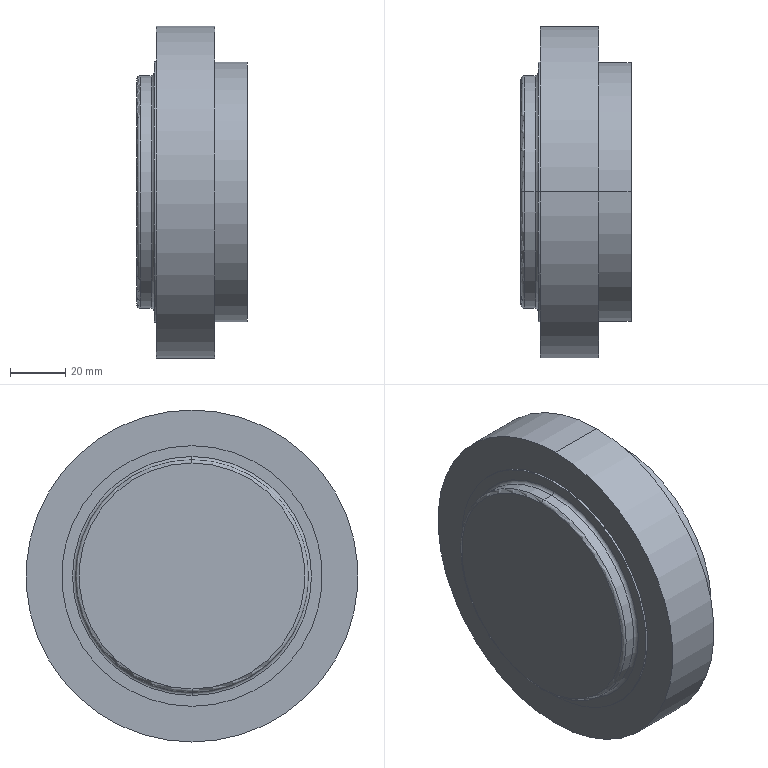Part | STEP file | Bearing end cap 1 | 1 solid | 26 faces | box 39.936 x 120.436 x 120.436 mm | volume 192561 mm3 | cylinder 10 | torus 6 | plane 6 | cone 4 | commonest cylinder face diameters 84.344 x2 87.483 x2 94.152 x2 94.544 x2 120.436 x2
STEP:
#1=CARTESIAN_POINT('',(-14.13,0.,40.292));
#2=VERTEX_POINT('',#1);
#3=CARTESIAN_POINT('',(-14.13,0.,-40.292));
#4=VERTEX_POINT('',#3);
#5=CARTESIAN_POINT('',(-14.13,0.,0.));
#6=DIRECTION('',(-1.,0.,0.));
#7=DIRECTION('',(0.,0.,1.));
#8=AXIS2_PLACEMENT_3D('',#5,#6,#7);
#9=CIRCLE('',#8,40.292);
#10=EDGE_CURVE('',#2,#4,#9,.T.);
#11=ORIENTED_EDGE('',*,*,#10,.F.);
#12=CARTESIAN_POINT('',(-15.049,0.,40.033));
#13=VERTEX_POINT('',#12);
#14=CARTESIAN_POINT('',(-15.644,0.,43.911));
#15=DIRECTION('',(0.,1.,0.));
#16=DIRECTION('',(0.,0.,1.));
#17=AXIS2_PLACEMENT_3D('',#14,#15,#16);
#18=CIRCLE('',#17,3.923);
#19=EDGE_CURVE('',#2,#13,#18,.T.);
#20=ORIENTED_EDGE('',*,*,#19,.T.);
#21=CARTESIAN_POINT('',(-15.049,0.,-40.033));
#22=VERTEX_POINT('',#21);
#23=CARTESIAN_POINT('',(-15.049,0.,0.));
#24=DIRECTION('',(1.,0.,0.));
#25=DIRECTION('',(0.,0.,1.));
#26=AXIS2_PLACEMENT_3D('',#23,#24,#25);
#27=CIRCLE('',#26,40.033);
#28=EDGE_CURVE('',#22,#13,#27,.T.);
#29=ORIENTED_EDGE('',*,*,#28,.F.);
#30=CARTESIAN_POINT('',(-15.644,0.,-43.911));
#31=DIRECTION('',(0.,-1.,0.));
#32=DIRECTION('',(0.,0.,-1.));
#33=AXIS2_PLACEMENT_3D('',#30,#31,#32);
#34=CIRCLE('',#33,3.923);
#35=EDGE_CURVE('',#4,#22,#34,.T.);
#36=ORIENTED_EDGE('',*,*,#35,.F.);
#37=EDGE_LOOP('',(#11,#20,#29,#36));
#38=FACE_OUTER_BOUND('',#37,.T.);
#39=CARTESIAN_POINT('',(-15.644,0.,0.));
#40=DIRECTION('',(1.,0.,0.));
#41=DIRECTION('',(0.,0.,-1.));
#42=AXIS2_PLACEMENT_3D('',#39,#40,#41);
#43=TOROIDAL_SURFACE('',#42,43.911,3.923);
#44=ADVANCED_FACE('',(#38),#43,.T.);
#45=CARTESIAN_POINT('',(-39.936,0.,40.995));
#46=VERTEX_POINT('',#45);
#47=CARTESIAN_POINT('',(-39.936,0.,-40.995));
#48=VERTEX_POINT('',#47);
#49=CARTESIAN_POINT('',(-39.936,0.,0.));
#50=DIRECTION('',(-1.,0.,0.));
#51=DIRECTION('',(0.,0.,-1.));
#52=AXIS2_PLACEMENT_3D('',#49,#50,#51);
#53=CIRCLE('',#52,40.995);
#54=EDGE_CURVE('',#46,#48,#53,.T.);
#55=ORIENTED_EDGE('',*,*,#54,.F.);
#56=CARTESIAN_POINT('',(-38.759,0.,42.172));
#57=VERTEX_POINT('',#56);
#58=CARTESIAN_POINT('',(-38.759,0.,40.995));
#59=DIRECTION('',(0.,1.,0.));
#60=DIRECTION('',(0.,0.,1.));
#61=AXIS2_PLACEMENT_3D('',#58,#59,#60);
#62=CIRCLE('',#61,1.177);
#63=EDGE_CURVE('',#46,#57,#62,.T.);
#64=ORIENTED_EDGE('',*,*,#63,.T.);
#65=CARTESIAN_POINT('',(-38.759,0.,-42.172));
#66=VERTEX_POINT('',#65);
#67=CARTESIAN_POINT('',(-38.759,0.,0.));
#68=DIRECTION('',(1.,0.,0.));
#69=DIRECTION('',(0.,0.,-1.));
#70=AXIS2_PLACEMENT_3D('',#67,#68,#69);
#71=CIRCLE('',#70,42.172);
#72=EDGE_CURVE('',#66,#57,#71,.T.);
#73=ORIENTED_EDGE('',*,*,#72,.F.);
#74=CARTESIAN_POINT('',(-38.759,0.,-40.995));
#75=DIRECTION('',(0.,-1.,0.));
#76=DIRECTION('',(0.,0.,-1.));
#77=AXIS2_PLACEMENT_3D('',#74,#75,#76);
#78=CIRCLE('',#77,1.177);
#79=EDGE_CURVE('',#48,#66,#78,.T.);
#80=ORIENTED_EDGE('',*,*,#79,.F.);
#81=EDGE_LOOP('',(#55,#64,#73,#80));
#82=FACE_OUTER_BOUND('',#81,.T.);
#83=CARTESIAN_POINT('',(-38.759,0.,0.));
#84=DIRECTION('',(1.,0.,0.));
#85=DIRECTION('',(0.,0.,-1.));
#86=AXIS2_PLACEMENT_3D('',#83,#84,#85);
#87=TOROIDAL_SURFACE('',#86,40.995,1.177);
#88=ADVANCED_FACE('',(#82),#87,.T.);
#89=CARTESIAN_POINT('',(-33.659,0.,43.349));
#90=VERTEX_POINT('',#89);
#91=CARTESIAN_POINT('',(-33.659,0.,-43.349));
#92=VERTEX_POINT('',#91);
#93=CARTESIAN_POINT('',(-33.659,0.,0.));
#94=DIRECTION('',(1.,0.,0.));
#95=DIRECTION('',(0.,0.,-1.));
#96=AXIS2_PLACEMENT_3D('',#93,#94,#95);
#97=CIRCLE('',#96,43.349);
#98=EDGE_CURVE('',#90,#92,#97,.T.);
#99=ORIENTED_EDGE('',*,*,#98,.F.);
#100=CARTESIAN_POINT('',(-34.836,0.,42.172));
#101=VERTEX_POINT('',#100);
#102=CARTESIAN_POINT('',(-34.836,0.,43.349));
#103=DIRECTION('',(0.,1.,0.));
#104=DIRECTION('',(0.,0.,1.));
#105=AXIS2_PLACEMENT_3D('',#102,#103,#104);
#106=CIRCLE('',#105,1.177);
#107=EDGE_CURVE('',#90,#101,#106,.T.);
#108=ORIENTED_EDGE('',*,*,#107,.T.);
#109=CARTESIAN_POINT('',(-34.836,0.,-42.172));
#110=VERTEX_POINT('',#109);
#111=CARTESIAN_POINT('',(-34.836,0.,0.));
#112=DIRECTION('',(-1.,0.,0.));
#113=DIRECTION('',(0.,0.,-1.));
#114=AXIS2_PLACEMENT_3D('',#111,#112,#113);
#115=CIRCLE('',#114,42.172);
#116=EDGE_CURVE('',#110,#101,#115,.T.);
#117=ORIENTED_EDGE('',*,*,#116,.F.);
#118=CARTESIAN_POINT('',(-34.836,0.,-43.349));
#119=DIRECTION('',(0.,-1.,0.));
#120=DIRECTION('',(0.,0.,-1.));
#121=AXIS2_PLACEMENT_3D('',#118,#119,#120);
#122=CIRCLE('',#121,1.177);
#123=EDGE_CURVE('',#92,#110,#122,.T.);
#124=ORIENTED_EDGE('',*,*,#123,.F.);
#125=EDGE_LOOP('',(#99,#108,#117,#124));
#126=FACE_OUTER_BOUND('',#125,.T.);
#127=CARTESIAN_POINT('',(-34.836,0.,0.));
#128=DIRECTION('',(1.,0.,0.));
#129=DIRECTION('',(0.,0.,-1.));
#130=AXIS2_PLACEMENT_3D('',#127,#128,#129);
#131=TOROIDAL_SURFACE('',#130,43.349,1.177);
#132=ADVANCED_FACE('',(#126),#131,.F.);
#133=CARTESIAN_POINT('',(-11.769,0.,60.218));
#134=VERTEX_POINT('',#133);
#135=CARTESIAN_POINT('',(-11.769,0.,-60.218));
#136=VERTEX_POINT('',#135);
#137=CARTESIAN_POINT('',(-11.769,0.,0.));
#138=DIRECTION('',(-1.,0.,0.));
#139=DIRECTION('',(0.,0.,1.));
#140=AXIS2_PLACEMENT_3D('',#137,#138,#139);
#141=CIRCLE('',#140,60.218);
#142=EDGE_CURVE('',#134,#136,#141,.T.);
#143=ORIENTED_EDGE('',*,*,#142,.T.);
#144=CARTESIAN_POINT('',(-32.875,0.,-60.218));
#145=VERTEX_POINT('',#144);
#146=CARTESIAN_POINT('',(0.,0.,-60.218));
#147=DIRECTION('',(-1.,0.,0.));
#148=VECTOR('',#147,1000.);
#149=LINE('',#146,#148);
#150=EDGE_CURVE('',#136,#145,#149,.T.);
#151=ORIENTED_EDGE('',*,*,#150,.T.);
#152=CARTESIAN_POINT('',(-32.875,0.,60.218));
#153=VERTEX_POINT('',#152);
#154=CARTESIAN_POINT('',(-32.875,0.,0.));
#155=DIRECTION('',(-1.,0.,0.));
#156=DIRECTION('',(0.,0.,1.));
#157=AXIS2_PLACEMENT_3D('',#154,#155,#156);
#158=CIRCLE('',#157,60.218);
#159=EDGE_CURVE('',#153,#145,#158,.T.);
#160=ORIENTED_EDGE('',*,*,#159,.F.);
#161=CARTESIAN_POINT('',(0.,0.,60.218));
#162=DIRECTION('',(-1.,0.,0.));
#163=VECTOR('',#162,1000.);
#164=LINE('',#161,#163);
#165=EDGE_CURVE('',#134,#153,#164,.T.);
#166=ORIENTED_EDGE('',*,*,#165,.F.);
#167=EDGE_LOOP('',(#143,#151,#160,#166));
#168=FACE_OUTER_BOUND('',#167,.T.);
#169=CARTESIAN_POINT('',(0.,0.,0.));
#170=DIRECTION('',(-1.,0.,0.));
#171=DIRECTION('',(0.,0.,1.));
#172=AXIS2_PLACEMENT_3D('',#169,#170,#171);
#173=CYLINDRICAL_SURFACE('',#172,60.218);
#174=ADVANCED_FACE('',(#168),#173,.T.);
#175=CARTESIAN_POINT('',(-32.875,0.,47.272));
#176=VERTEX_POINT('',#175);
#177=CARTESIAN_POINT('',(-32.875,0.,-47.272));
#178=VERTEX_POINT('',#177);
#179=CARTESIAN_POINT('',(-32.875,0.,0.));
#180=DIRECTION('',(-1.,0.,0.));
#181=DIRECTION('',(0.,0.,1.));
#182=AXIS2_PLACEMENT_3D('',#179,#180,#181);
#183=CIRCLE('',#182,47.272);
#184=EDGE_CURVE('',#176,#178,#183,.T.);
#185=ORIENTED_EDGE('',*,*,#184,.T.);
#186=CARTESIAN_POINT('',(-33.659,0.,-47.272));
#187=VERTEX_POINT('',#186);
#188=CARTESIAN_POINT('',(0.,0.,-47.272));
#189=DIRECTION('',(-1.,0.,0.));
#190=VECTOR('',#189,1000.);
#191=LINE('',#188,#190);
#192=EDGE_CURVE('',#178,#187,#191,.T.);
#193=ORIENTED_EDGE('',*,*,#192,.T.);
#194=CARTESIAN_POINT('',(-33.659,0.,47.272));
#195=VERTEX_POINT('',#194);
#196=CARTESIAN_POINT('',(-33.659,0.,0.));
#197=DIRECTION('',(-1.,0.,0.));
#198=DIRECTION('',(0.,0.,1.));
#199=AXIS2_PLACEMENT_3D('',#196,#197,#198);
#200=CIRCLE('',#199,47.272);
#201=EDGE_CURVE('',#195,#187,#200,.T.);
#202=ORIENTED_EDGE('',*,*,#201,.F.);
#203=CARTESIAN_POINT('',(0.,0.,47.272));
#204=DIRECTION('',(-1.,0.,0.));
#205=VECTOR('',#204,1000.);
#206=LINE('',#203,#205);
#207=EDGE_CURVE('',#176,#195,#206,.T.);
#208=ORIENTED_EDGE('',*,*,#207,.F.);
#209=EDGE_LOOP('',(#185,#193,#202,#208));
#210=FACE_OUTER_BOUND('',#209,.T.);
#211=CARTESIAN_POINT('',(0.,0.,0.));
#212=DIRECTION('',(-1.,0.,0.));
#213=DIRECTION('',(0.,0.,1.));
#214=AXIS2_PLACEMENT_3D('',#211,#212,#213);
#215=CYLINDRICAL_SURFACE('',#214,47.272);
#216=ADVANCED_FACE('',(#210),#215,.T.);
#217=CARTESIAN_POINT('',(-34.836,0.,0.));
#218=DIRECTION('',(-1.,0.,0.));
#219=DIRECTION('',(0.,0.,-1.));
#220=AXIS2_PLACEMENT_3D('',#217,#218,#219);
#221=CIRCLE('',#220,42.172);
#222=EDGE_CURVE('',#101,#110,#221,.T.);
#223=ORIENTED_EDGE('',*,*,#222,.T.);
#224=CARTESIAN_POINT('',(0.,0.,-42.172));
#225=DIRECTION('',(-1.,0.,0.));
#226=VECTOR('',#225,1000.);
#227=LINE('',#224,#226);
#228=EDGE_CURVE('',#110,#66,#227,.T.);
#229=ORIENTED_EDGE('',*,*,#228,.T.);
#230=ORIENTED_EDGE('',*,*,#72,.T.);
#231=CARTESIAN_POINT('',(0.,0.,42.172));
#232=DIRECTION('',(-1.,0.,0.));
#233=VECTOR('',#232,1000.);
#234=LINE('',#231,#233);
#235=EDGE_CURVE('',#101,#57,#234,.T.);
#236=ORIENTED_EDGE('',*,*,#235,.F.);
#237=EDGE_LOOP('',(#223,#229,#230,#236));
#238=FACE_OUTER_BOUND('',#237,.T.);
#239=CARTESIAN_POINT('',(0.,0.,0.));
#240=DIRECTION('',(-1.,0.,0.));
#241=DIRECTION('',(0.,0.,1.));
#242=AXIS2_PLACEMENT_3D('',#239,#240,#241);
#243=CYLINDRICAL_SURFACE('',#242,42.172);
#244=ADVANCED_FACE('',(#238),#243,.T.);
#245=CARTESIAN_POINT('',(-33.071,0.,-37.268));
#246=VERTEX_POINT('',#245);
#247=CARTESIAN_POINT('',(-33.071,0.,37.268));
#248=VERTEX_POINT('',#247);
#249=CARTESIAN_POINT('',(-33.071,0.,0.));
#250=DIRECTION('',(-1.,0.,0.));
#251=DIRECTION('',(0.,0.,1.));
#252=AXIS2_PLACEMENT_3D('',#249,#250,#251);
#253=CIRCLE('',#252,37.268);
#254=EDGE_CURVE('',#246,#248,#253,.T.);
#255=ORIENTED_EDGE('',*,*,#254,.T.);
#256=CARTESIAN_POINT('',(-33.071,0.,37.268));
#257=DIRECTION('',(0.9884,0.,0.1516));
#258=VECTOR('',#257,1000.);
#259=LINE('',#256,#258);
#260=EDGE_CURVE('',#248,#13,#259,.T.);
#261=ORIENTED_EDGE('',*,*,#260,.T.);
#262=CARTESIAN_POINT('',(-15.049,0.,0.));
#263=DIRECTION('',(1.,0.,0.));
#264=DIRECTION('',(0.,0.,1.));
#265=AXIS2_PLACEMENT_3D('',#262,#263,#264);
#266=CIRCLE('',#265,40.033);
#267=EDGE_CURVE('',#13,#22,#266,.T.);
#268=ORIENTED_EDGE('',*,*,#267,.T.);
#269=CARTESIAN_POINT('',(-33.071,0.,-37.268));
#270=DIRECTION('',(0.9884,0.,-0.1516));
#271=VECTOR('',#270,1000.);
#272=LINE('',#269,#271);
#273=EDGE_CURVE('',#246,#22,#272,.T.);
#274=ORIENTED_EDGE('',*,*,#273,.F.);
#275=EDGE_LOOP('',(#255,#261,#268,#274));
#276=FACE_OUTER_BOUND('',#275,.T.);
#277=CARTESIAN_POINT('',(-33.071,0.,0.));
#278=DIRECTION('',(1.,0.,0.));
#279=DIRECTION('',(0.,0.,-1.));
#280=AXIS2_PLACEMENT_3D('',#277,#278,#279);
#281=CONICAL_SURFACE('',#280,37.268,0.1522);
#282=ADVANCED_FACE('',(#276),#281,.F.);
#283=CARTESIAN_POINT('',(-14.13,0.,0.));
#284=DIRECTION('',(-1.,0.,0.));
#285=DIRECTION('',(0.,0.,1.));
#286=AXIS2_PLACEMENT_3D('',#283,#284,#285);
#287=CIRCLE('',#286,40.292);
#288=EDGE_CURVE('',#4,#2,#287,.T.);
#289=ORIENTED_EDGE('',*,*,#288,.T.);
#290=CARTESIAN_POINT('',(-5.884,0.,43.741));
#291=VERTEX_POINT('',#290);
#292=CARTESIAN_POINT('',(-14.574,0.,40.106));
#293=DIRECTION('',(0.9225,0.,0.386));
#294=VECTOR('',#293,1000.);
#295=LINE('',#292,#294);
#296=EDGE_CURVE('',#2,#291,#295,.T.);
#297=ORIENTED_EDGE('',*,*,#296,.T.);
#298=CARTESIAN_POINT('',(-5.884,0.,-43.741));
#299=VERTEX_POINT('',#298);
#300=CARTESIAN_POINT('',(-5.884,0.,0.));
#301=DIRECTION('',(-1.,0.,0.));
#302=DIRECTION('',(0.,0.,1.));
#303=AXIS2_PLACEMENT_3D('',#300,#301,#302);
#304=CIRCLE('',#303,43.741);
#305=EDGE_CURVE('',#299,#291,#304,.T.);
#306=ORIENTED_EDGE('',*,*,#305,.F.);
#307=CARTESIAN_POINT('',(-14.574,0.,-40.106));
#308=DIRECTION('',(0.9225,0.,-0.386));
#309=VECTOR('',#308,1000.);
#310=LINE('',#307,#309);
#311=EDGE_CURVE('',#4,#299,#310,.T.);
#312=ORIENTED_EDGE('',*,*,#311,.F.);
#313=EDGE_LOOP('',(#289,#297,#306,#312));
#314=FACE_OUTER_BOUND('',#313,.T.);
#315=CARTESIAN_POINT('',(-14.574,0.,0.));
#316=DIRECTION('',(1.,0.,0.));
#317=DIRECTION('',(0.,0.,-1.));
#318=AXIS2_PLACEMENT_3D('',#315,#316,#317);
#319=CONICAL_SURFACE('',#318,40.106,0.3962);
#320=ADVANCED_FACE('',(#314),#319,.F.);
#321=CARTESIAN_POINT('',(0.,0.,-43.741));
#322=VERTEX_POINT('',#321);
#323=CARTESIAN_POINT('',(0.,0.,43.741));
#324=VERTEX_POINT('',#323);
#325=CARTESIAN_POINT('',(0.,0.,0.));
#326=DIRECTION('',(-1.,0.,0.));
#327=DIRECTION('',(0.,0.,1.));
#328=AXIS2_PLACEMENT_3D('',#325,#326,#327);
#329=CIRCLE('',#328,43.741);
#330=EDGE_CURVE('',#322,#324,#329,.T.);
#331=ORIENTED_EDGE('',*,*,#330,.F.);
#332=CARTESIAN_POINT('',(0.,0.,-43.741));
#333=DIRECTION('',(-1.,0.,0.));
#334=VECTOR('',#333,1000.);
#335=LINE('',#332,#334);
#336=EDGE_CURVE('',#322,#299,#335,.T.);
#337=ORIENTED_EDGE('',*,*,#336,.T.);
#338=ORIENTED_EDGE('',*,*,#305,.T.);
#339=CARTESIAN_POINT('',(0.,0.,43.741));
#340=DIRECTION('',(-1.,0.,0.));
#341=VECTOR('',#340,1000.);
#342=LINE('',#339,#341);
#343=EDGE_CURVE('',#324,#291,#342,.T.);
#344=ORIENTED_EDGE('',*,*,#343,.F.);
#345=EDGE_LOOP('',(#331,#337,#338,#344));
#346=FACE_OUTER_BOUND('',#345,.T.);
#347=CARTESIAN_POINT('',(0.,0.,0.));
#348=DIRECTION('',(-1.,0.,0.));
#349=DIRECTION('',(0.,0.,1.));
#350=AXIS2_PLACEMENT_3D('',#347,#348,#349);
#351=CYLINDRICAL_SURFACE('',#350,43.741);
#352=ADVANCED_FACE('',(#346),#351,.F.);
#353=CARTESIAN_POINT('',(0.,0.,47.076));
#354=VERTEX_POINT('',#353);
#355=CARTESIAN_POINT('',(0.,0.,-47.076));
#356=VERTEX_POINT('',#355);
#357=CARTESIAN_POINT('',(0.,0.,0.));
#358=DIRECTION('',(-1.,0.,0.));
#359=DIRECTION('',(0.,0.,1.));
#360=AXIS2_PLACEMENT_3D('',#357,#358,#359);
#361=CIRCLE('',#360,47.076);
#362=EDGE_CURVE('',#354,#356,#361,.T.);
#363=ORIENTED_EDGE('',*,*,#362,.T.);
#364=CARTESIAN_POINT('',(-11.769,0.,-47.076));
#365=VERTEX_POINT('',#364);
#366=CARTESIAN_POINT('',(0.,0.,-47.076));
#367=DIRECTION('',(-1.,0.,0.));
#368=VECTOR('',#367,1000.);
#369=LINE('',#366,#368);
#370=EDGE_CURVE('',#356,#365,#369,.T.);
#371=ORIENTED_EDGE('',*,*,#370,.T.);
#372=CARTESIAN_POINT('',(-11.769,0.,47.076));
#373=VERTEX_POINT('',#372);
#374=CARTESIAN_POINT('',(-11.769,0.,0.));
#375=DIRECTION('',(-1.,0.,0.));
#376=DIRECTION('',(0.,0.,1.));
#377=AXIS2_PLACEMENT_3D('',#374,#375,#376);
#378=CIRCLE('',#377,47.076);
#379=EDGE_CURVE('',#373,#365,#378,.T.);
#380=ORIENTED_EDGE('',*,*,#379,.F.);
#381=CARTESIAN_POINT('',(0.,0.,47.076));
#382=DIRECTION('',(-1.,0.,0.));
#383=VECTOR('',#382,1000.);
#384=LINE('',#381,#383);
#385=EDGE_CURVE('',#354,#373,#384,.T.);
#386=ORIENTED_EDGE('',*,*,#385,.F.);
#387=EDGE_LOOP('',(#363,#371,#380,#386));
#388=FACE_OUTER_BOUND('',#387,.T.);
#389=CARTESIAN_POINT('',(0.,0.,0.));
#390=DIRECTION('',(-1.,0.,0.));
#391=DIRECTION('',(0.,0.,1.));
#392=AXIS2_PLACEMENT_3D('',#389,#390,#391);
#393=CYLINDRICAL_SURFACE('',#392,47.076);
#394=ADVANCED_FACE('',(#388),#393,.T.);
#395=ORIENTED_EDGE('',*,*,#370,.F.);
#396=CARTESIAN_POINT('',(0.,0.,0.));
#397=DIRECTION('',(-1.,0.,0.));
#398=DIRECTION('',(0.,0.,1.));
#399=AXIS2_PLACEMENT_3D('',#396,#397,#398);
#400=CIRCLE('',#399,47.076);
#401=EDGE_CURVE('',#356,#354,#400,.T.);
#402=ORIENTED_EDGE('',*,*,#401,.T.);
#403=ORIENTED_EDGE('',*,*,#385,.T.);
#404=CARTESIAN_POINT('',(-11.769,0.,0.));
#405=DIRECTION('',(-1.,0.,0.));
#406=DIRECTION('',(0.,0.,1.));
#407=AXIS2_PLACEMENT_3D('',#404,#405,#406);
#408=CIRCLE('',#407,47.076);
#409=EDGE_CURVE('',#365,#373,#408,.T.);
#410=ORIENTED_EDGE('',*,*,#409,.F.);
#411=EDGE_LOOP('',(#395,#402,#403,#410));
#412=FACE_OUTER_BOUND('',#411,.T.);
#413=CARTESIAN_POINT('',(0.,0.,0.));
#414=DIRECTION('',(-1.,0.,0.));
#415=DIRECTION('',(0.,0.,1.));
#416=AXIS2_PLACEMENT_3D('',#413,#414,#415);
#417=CYLINDRICAL_SURFACE('',#416,47.076);
#418=ADVANCED_FACE('',(#412),#417,.T.);
#419=ORIENTED_EDGE('',*,*,#362,.F.);
#420=ORIENTED_EDGE('',*,*,#401,.F.);
#421=EDGE_LOOP('',(#419,#420));
#422=FACE_OUTER_BOUND('',#421,.T.);
#423=CARTESIAN_POINT('',(0.,0.,0.));
#424=DIRECTION('',(-1.,0.,0.));
#425=DIRECTION('',(0.,0.,1.));
#426=AXIS2_PLACEMENT_3D('',#423,#424,#425);
#427=CIRCLE('',#426,43.741);
#428=EDGE_CURVE('',#324,#322,#427,.T.);
#429=ORIENTED_EDGE('',*,*,#428,.T.);
#430=ORIENTED_EDGE('',*,*,#330,.T.);
#431=EDGE_LOOP('',(#429,#430));
#432=FACE_BOUND('',#431,.T.);
#433=CARTESIAN_POINT('',(0.,47.076,0.));
#434=DIRECTION('',(-1.,0.,0.));
#435=DIRECTION('',(0.,0.,1.));
#436=AXIS2_PLACEMENT_3D('',#433,#434,#435);
#437=PLANE('',#436);
#438=ADVANCED_FACE('',(#422,#432),#437,.F.);
#439=ORIENTED_EDGE('',*,*,#336,.F.);
#440=ORIENTED_EDGE('',*,*,#428,.F.);
#441=ORIENTED_EDGE('',*,*,#343,.T.);
#442=CARTESIAN_POINT('',(-5.884,0.,0.));
#443=DIRECTION('',(-1.,0.,0.));
#444=DIRECTION('',(0.,0.,1.));
#445=AXIS2_PLACEMENT_3D('',#442,#443,#444);
#446=CIRCLE('',#445,43.741);
#447=EDGE_CURVE('',#291,#299,#446,.T.);
#448=ORIENTED_EDGE('',*,*,#447,.T.);
#449=EDGE_LOOP('',(#439,#440,#441,#448));
#450=FACE_OUTER_BOUND('',#449,.T.);
#451=CARTESIAN_POINT('',(0.,0.,0.));
#452=DIRECTION('',(-1.,0.,0.));
#453=DIRECTION('',(0.,0.,1.));
#454=AXIS2_PLACEMENT_3D('',#451,#452,#453);
#455=CYLINDRICAL_SURFACE('',#454,43.741);
#456=ADVANCED_FACE('',(#450),#455,.F.);
#457=ORIENTED_EDGE('',*,*,#296,.F.);
#458=ORIENTED_EDGE('',*,*,#10,.T.);
#459=ORIENTED_EDGE('',*,*,#311,.T.);
#460=ORIENTED_EDGE('',*,*,#447,.F.);
#461=EDGE_LOOP('',(#457,#458,#459,#460));
#462=FACE_OUTER_BOUND('',#461,.T.);
#463=CARTESIAN_POINT('',(-14.574,0.,0.));
#464=DIRECTION('',(1.,0.,0.));
#465=DIRECTION('',(0.,0.,-1.));
#466=AXIS2_PLACEMENT_3D('',#463,#464,#465);
#467=CONICAL_SURFACE('',#466,40.106,0.3962);
#468=ADVANCED_FACE('',(#462),#467,.F.);
#469=ORIENTED_EDGE('',*,*,#260,.F.);
#470=CARTESIAN_POINT('',(-33.071,0.,0.));
#471=DIRECTION('',(-1.,0.,0.));
#472=DIRECTION('',(0.,0.,1.));
#473=AXIS2_PLACEMENT_3D('',#470,#471,#472);
#474=CIRCLE('',#473,37.268);
#475=EDGE_CURVE('',#248,#246,#474,.T.);
#476=ORIENTED_EDGE('',*,*,#475,.T.);
#477=ORIENTED_EDGE('',*,*,#273,.T.);
#478=ORIENTED_EDGE('',*,*,#28,.T.);
#479=EDGE_LOOP('',(#469,#476,#477,#478));
#480=FACE_OUTER_BOUND('',#479,.T.);
#481=CARTESIAN_POINT('',(-33.071,0.,0.));
#482=DIRECTION('',(1.,0.,0.));
#483=DIRECTION('',(0.,0.,-1.));
#484=AXIS2_PLACEMENT_3D('',#481,#482,#483);
#485=CONICAL_SURFACE('',#484,37.268,0.1522);
#486=ADVANCED_FACE('',(#480),#485,.F.);
#487=ORIENTED_EDGE('',*,*,#254,.F.);
#488=ORIENTED_EDGE('',*,*,#475,.F.);
#489=EDGE_LOOP('',(#487,#488));
#490=FACE_OUTER_BOUND('',#489,.T.);
#491=CARTESIAN_POINT('',(-33.071,0.,0.));
#492=DIRECTION('',(-1.,0.,0.));
#493=DIRECTION('',(0.,0.,1.));
#494=AXIS2_PLACEMENT_3D('',#491,#492,#493);
#495=PLANE('',#494);
#496=ADVANCED_FACE('',(#490),#495,.F.);
#497=CARTESIAN_POINT('',(-39.936,0.,0.));
#498=DIRECTION('',(-1.,0.,0.));
#499=DIRECTION('',(0.,0.,-1.));
#500=AXIS2_PLACEMENT_3D('',#497,#498,#499);
#501=CIRCLE('',#500,40.995);
#502=EDGE_CURVE('',#48,#46,#501,.T.);
#503=ORIENTED_EDGE('',*,*,#502,.T.);
#504=ORIENTED_EDGE('',*,*,#54,.T.);
#505=EDGE_LOOP('',(#503,#504));
#506=FACE_OUTER_BOUND('',#505,.T.);
#507=CARTESIAN_POINT('',(-39.936,42.172,0.));
#508=DIRECTION('',(1.,0.,0.));
#509=DIRECTION('',(0.,0.,-1.));
#510=AXIS2_PLACEMENT_3D('',#507,#508,#509);
#511=PLANE('',#510);
#512=ADVANCED_FACE('',(#506),#511,.F.);
#513=ORIENTED_EDGE('',*,*,#228,.F.);
#514=ORIENTED_EDGE('',*,*,#116,.T.);
#515=ORIENTED_EDGE('',*,*,#235,.T.);
#516=CARTESIAN_POINT('',(-38.759,0.,0.));
#517=DIRECTION('',(1.,0.,0.));
#518=DIRECTION('',(0.,0.,-1.));
#519=AXIS2_PLACEMENT_3D('',#516,#517,#518);
#520=CIRCLE('',#519,42.172);
#521=EDGE_CURVE('',#57,#66,#520,.T.);
#522=ORIENTED_EDGE('',*,*,#521,.T.);
#523=EDGE_LOOP('',(#513,#514,#515,#522));
#524=FACE_OUTER_BOUND('',#523,.T.);
#525=CARTESIAN_POINT('',(0.,0.,0.));
#526=DIRECTION('',(-1.,0.,0.));
#527=DIRECTION('',(0.,0.,1.));
#528=AXIS2_PLACEMENT_3D('',#525,#526,#527);
#529=CYLINDRICAL_SURFACE('',#528,42.172);
#530=ADVANCED_FACE('',(#524),#529,.T.);
#531=CARTESIAN_POINT('',(-33.659,0.,0.));
#532=DIRECTION('',(1.,0.,0.));
#533=DIRECTION('',(0.,0.,-1.));
#534=AXIS2_PLACEMENT_3D('',#531,#532,#533);
#535=CIRCLE('',#534,43.349);
#536=EDGE_CURVE('',#92,#90,#535,.T.);
#537=ORIENTED_EDGE('',*,*,#536,.T.);
#538=ORIENTED_EDGE('',*,*,#98,.T.);
#539=EDGE_LOOP('',(#537,#538));
#540=FACE_BOUND('',#539,.T.);
#541=ORIENTED_EDGE('',*,*,#201,.T.);
#542=CARTESIAN_POINT('',(-33.659,0.,0.));
#543=DIRECTION('',(-1.,0.,0.));
#544=DIRECTION('',(0.,0.,1.));
#545=AXIS2_PLACEMENT_3D('',#542,#543,#544);
#546=CIRCLE('',#545,47.272);
#547=EDGE_CURVE('',#187,#195,#546,.T.);
#548=ORIENTED_EDGE('',*,*,#547,.T.);
#549=EDGE_LOOP('',(#541,#548));
#550=FACE_OUTER_BOUND('',#549,.T.);
#551=CARTESIAN_POINT('',(-33.659,47.272,0.));
#552=DIRECTION('',(1.,0.,0.));
#553=DIRECTION('',(0.,0.,-1.));
#554=AXIS2_PLACEMENT_3D('',#551,#552,#553);
#555=PLANE('',#554);
#556=ADVANCED_FACE('',(#540,#550),#555,.F.);
#557=ORIENTED_EDGE('',*,*,#192,.F.);
#558=CARTESIAN_POINT('',(-32.875,0.,0.));
#559=DIRECTION('',(-1.,0.,0.));
#560=DIRECTION('',(0.,0.,1.));
#561=AXIS2_PLACEMENT_3D('',#558,#559,#560);
#562=CIRCLE('',#561,47.272);
#563=EDGE_CURVE('',#178,#176,#562,.T.);
#564=ORIENTED_EDGE('',*,*,#563,.T.);
#565=ORIENTED_EDGE('',*,*,#207,.T.);
#566=ORIENTED_EDGE('',*,*,#547,.F.);
#567=EDGE_LOOP('',(#557,#564,#565,#566));
#568=FACE_OUTER_BOUND('',#567,.T.);
#569=CARTESIAN_POINT('',(0.,0.,0.));
#570=DIRECTION('',(-1.,0.,0.));
#571=DIRECTION('',(0.,0.,1.));
#572=AXIS2_PLACEMENT_3D('',#569,#570,#571);
#573=CYLINDRICAL_SURFACE('',#572,47.272);
#574=ADVANCED_FACE('',(#568),#573,.T.);
#575=ORIENTED_EDGE('',*,*,#184,.F.);
#576=ORIENTED_EDGE('',*,*,#563,.F.);
#577=EDGE_LOOP('',(#575,#576));
#578=FACE_BOUND('',#577,.T.);
#579=ORIENTED_EDGE('',*,*,#159,.T.);
#580=CARTESIAN_POINT('',(-32.875,0.,0.));
#581=DIRECTION('',(-1.,0.,0.));
#582=DIRECTION('',(0.,0.,1.));
#583=AXIS2_PLACEMENT_3D('',#580,#581,#582);
#584=CIRCLE('',#583,60.218);
#585=EDGE_CURVE('',#145,#153,#584,.T.);
#586=ORIENTED_EDGE('',*,*,#585,.T.);
#587=EDGE_LOOP('',(#579,#586));
#588=FACE_OUTER_BOUND('',#587,.T.);
#589=CARTESIAN_POINT('',(-32.875,60.218,0.));
#590=DIRECTION('',(1.,0.,0.));
#591=DIRECTION('',(0.,0.,-1.));
#592=AXIS2_PLACEMENT_3D('',#589,#590,#591);
#593=PLANE('',#592);
#594=ADVANCED_FACE('',(#578,#588),#593,.F.);
#595=ORIENTED_EDGE('',*,*,#150,.F.);
#596=CARTESIAN_POINT('',(-11.769,0.,0.));
#597=DIRECTION('',(-1.,0.,0.));
#598=DIRECTION('',(0.,0.,1.));
#599=AXIS2_PLACEMENT_3D('',#596,#597,#598);
#600=CIRCLE('',#599,60.218);
#601=EDGE_CURVE('',#136,#134,#600,.T.);
#602=ORIENTED_EDGE('',*,*,#601,.T.);
#603=ORIENTED_EDGE('',*,*,#165,.T.);
#604=ORIENTED_EDGE('',*,*,#585,.F.);
#605=EDGE_LOOP('',(#595,#602,#603,#604));
#606=FACE_OUTER_BOUND('',#605,.T.);
#607=CARTESIAN_POINT('',(0.,0.,0.));
#608=DIRECTION('',(-1.,0.,0.));
#609=DIRECTION('',(0.,0.,1.));
#610=AXIS2_PLACEMENT_3D('',#607,#608,#609);
#611=CYLINDRICAL_SURFACE('',#610,60.218);
#612=ADVANCED_FACE('',(#606),#611,.T.);
#613=ORIENTED_EDGE('',*,*,#142,.F.);
#614=ORIENTED_EDGE('',*,*,#601,.F.);
#615=EDGE_LOOP('',(#613,#614));
#616=FACE_OUTER_BOUND('',#615,.T.);
#617=ORIENTED_EDGE('',*,*,#379,.T.);
#618=ORIENTED_EDGE('',*,*,#409,.T.);
#619=EDGE_LOOP('',(#617,#618));
#620=FACE_BOUND('',#619,.T.);
#621=CARTESIAN_POINT('',(-11.769,47.076,0.));
#622=DIRECTION('',(-1.,0.,0.));
#623=DIRECTION('',(0.,0.,1.));
#624=AXIS2_PLACEMENT_3D('',#621,#622,#623);
#625=PLANE('',#624);
#626=ADVANCED_FACE('',(#616,#620),#625,.F.);
#627=ORIENTED_EDGE('',*,*,#107,.F.);
#628=ORIENTED_EDGE('',*,*,#536,.F.);
#629=ORIENTED_EDGE('',*,*,#123,.T.);
#630=ORIENTED_EDGE('',*,*,#222,.F.);
#631=EDGE_LOOP('',(#627,#628,#629,#630));
#632=FACE_OUTER_BOUND('',#631,.T.);
#633=CARTESIAN_POINT('',(-34.836,0.,0.));
#634=DIRECTION('',(1.,0.,0.));
#635=DIRECTION('',(0.,0.,-1.));
#636=AXIS2_PLACEMENT_3D('',#633,#634,#635);
#637=TOROIDAL_SURFACE('',#636,43.349,1.177);
#638=ADVANCED_FACE('',(#632),#637,.F.);
#639=ORIENTED_EDGE('',*,*,#63,.F.);
#640=ORIENTED_EDGE('',*,*,#502,.F.);
#641=ORIENTED_EDGE('',*,*,#79,.T.);
#642=ORIENTED_EDGE('',*,*,#521,.F.);
#643=EDGE_LOOP('',(#639,#640,#641,#642));
#644=FACE_OUTER_BOUND('',#643,.T.);
#645=CARTESIAN_POINT('',(-38.759,0.,0.));
#646=DIRECTION('',(1.,0.,0.));
#647=DIRECTION('',(0.,0.,-1.));
#648=AXIS2_PLACEMENT_3D('',#645,#646,#647);
#649=TOROIDAL_SURFACE('',#648,40.995,1.177);
#650=ADVANCED_FACE('',(#644),#649,.T.);
#651=ORIENTED_EDGE('',*,*,#19,.F.);
#652=ORIENTED_EDGE('',*,*,#288,.F.);
#653=ORIENTED_EDGE('',*,*,#35,.T.);
#654=ORIENTED_EDGE('',*,*,#267,.F.);
#655=EDGE_LOOP('',(#651,#652,#653,#654));
#656=FACE_OUTER_BOUND('',#655,.T.);
#657=CARTESIAN_POINT('',(-15.644,0.,0.));
#658=DIRECTION('',(1.,0.,0.));
#659=DIRECTION('',(0.,0.,-1.));
#660=AXIS2_PLACEMENT_3D('',#657,#658,#659);
#661=TOROIDAL_SURFACE('',#660,43.911,3.923);
#662=ADVANCED_FACE('',(#656),#661,.T.);
#663=CLOSED_SHELL('',(#44,#88,#132,#174,#216,#244,#282,#320,#352,#394,#418,#438,#456,#468,#486,#496,#512,#530,#556,#574,#594,#612,#626,#638,#650,#662));
#664=MANIFOLD_SOLID_BREP('',#663);
#665=CARTESIAN_POINT('',(0.,0.,0.));
#666=DIRECTION('',(0.,0.,1.));
#667=DIRECTION('',(1.,0.,0.));
#668=AXIS2_PLACEMENT_3D('',#665,#666,#667);
#669=(LENGTH_UNIT()NAMED_UNIT(*)SI_UNIT(.MILLI.,.METRE.));
#670=UNCERTAINTY_MEASURE_WITH_UNIT(LENGTH_MEASURE(0.00001),#669,'','');
#671=(NAMED_UNIT(*)PLANE_ANGLE_UNIT()SI_UNIT($,.RADIAN.));
#672=(NAMED_UNIT(*)SI_UNIT($,.STERADIAN.)SOLID_ANGLE_UNIT());
#673=(GEOMETRIC_REPRESENTATION_CONTEXT(3)GLOBAL_UNCERTAINTY_ASSIGNED_CONTEXT((#670))GLOBAL_UNIT_ASSIGNED_CONTEXT((#669,#671,#672))REPRESENTATION_CONTEXT('',''));
#674=ADVANCED_BREP_SHAPE_REPRESENTATION('',(#664,#668),#673);